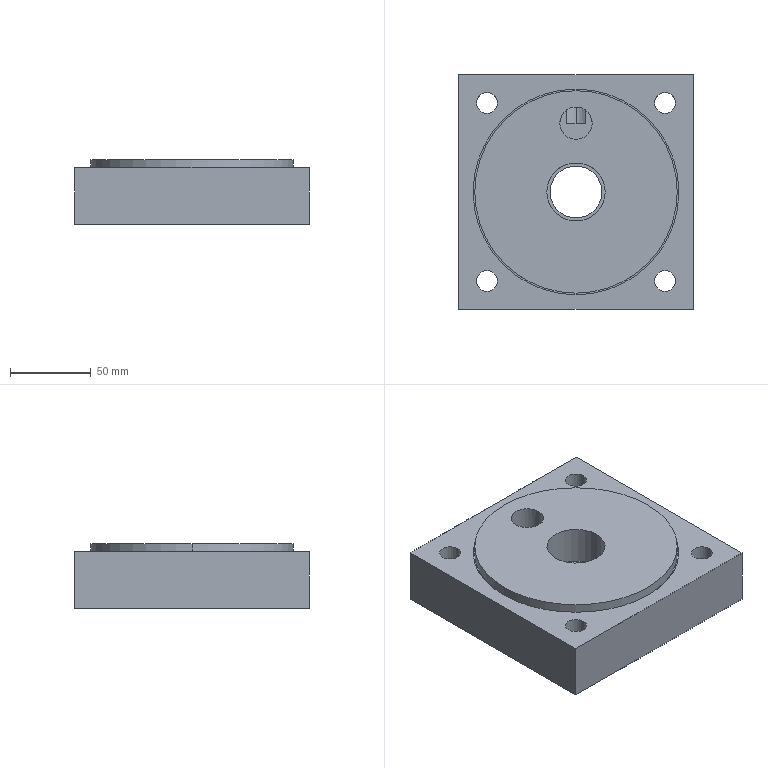Part | SolidWorks | features BaseBody 1, Cut 1 | 1 solid | 61 faces | box 145 x 145 x 40 mm | volume 721249 mm3 | cylinder 41 | plane 15 | spline 5 | commonest cylinder face diameters 19 x17 13 x8 32 x4 20 x2 24.478 x2 36 x2